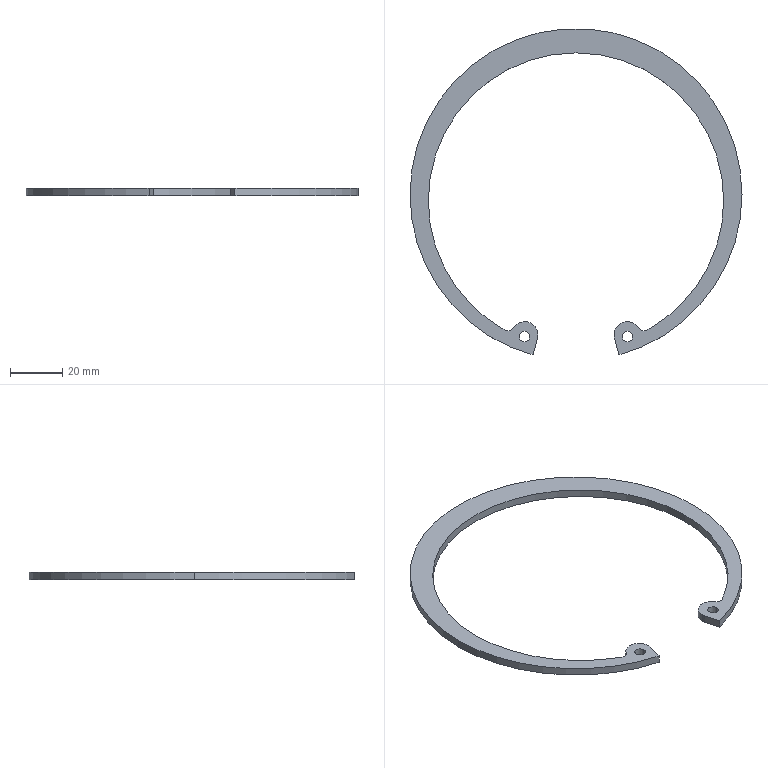Part | SolidWorks | features Extrusion 1 | 1 solid | 19 faces | box 127 x 124.836 x 3 mm | volume 7725 mm3 | cylinder 15 | plane 4 | commonest cylinder face diameters 4 x4 10 x3 113 x3 127 x3 5 x2
STEP:
#1=CARTESIAN_POINT('',(17.733,-54.327,1.5));
#2=VERTEX_POINT('',#1);
#3=CARTESIAN_POINT('',(21.733,-54.327,1.5));
#4=VERTEX_POINT('',#3);
#5=CARTESIAN_POINT('',(19.733,-54.327,1.5));
#6=DIRECTION('',(0.,0.,1.));
#7=DIRECTION('',(-1.,0.,0.));
#8=AXIS2_PLACEMENT_3D('',#5,#6,#7);
#9=CIRCLE('',#8,2.);
#10=EDGE_CURVE('',#2,#4,#9,.T.);
#11=ORIENTED_EDGE('',*,*,#10,.T.);
#12=CARTESIAN_POINT('',(21.733,-54.327,-1.5));
#13=VERTEX_POINT('',#12);
#14=CARTESIAN_POINT('',(21.733,-54.327,1.5));
#15=DIRECTION('',(0.,0.,-1.));
#16=VECTOR('',#15,1000.);
#17=LINE('',#14,#16);
#18=EDGE_CURVE('',#4,#13,#17,.T.);
#19=ORIENTED_EDGE('',*,*,#18,.T.);
#20=CARTESIAN_POINT('',(17.733,-54.327,-1.5));
#21=VERTEX_POINT('',#20);
#22=CARTESIAN_POINT('',(19.733,-54.327,-1.5));
#23=DIRECTION('',(0.,0.,1.));
#24=DIRECTION('',(-1.,0.,0.));
#25=AXIS2_PLACEMENT_3D('',#22,#23,#24);
#26=CIRCLE('',#25,2.);
#27=EDGE_CURVE('',#21,#13,#26,.T.);
#28=ORIENTED_EDGE('',*,*,#27,.F.);
#29=CARTESIAN_POINT('',(17.733,-54.327,1.5));
#30=DIRECTION('',(0.,0.,-1.));
#31=VECTOR('',#30,1000.);
#32=LINE('',#29,#31);
#33=EDGE_CURVE('',#2,#21,#32,.T.);
#34=ORIENTED_EDGE('',*,*,#33,.F.);
#35=EDGE_LOOP('',(#11,#19,#28,#34));
#36=FACE_OUTER_BOUND('',#35,.T.);
#37=CARTESIAN_POINT('',(19.733,-54.327,1.5));
#38=DIRECTION('',(0.,0.,-1.));
#39=DIRECTION('',(-1.,0.,0.));
#40=AXIS2_PLACEMENT_3D('',#37,#38,#39);
#41=CYLINDRICAL_SURFACE('',#40,2.);
#42=ADVANCED_FACE('',(#36),#41,.F.);
#43=CARTESIAN_POINT('',(-21.733,-54.327,1.5));
#44=VERTEX_POINT('',#43);
#45=CARTESIAN_POINT('',(-17.733,-54.327,1.5));
#46=VERTEX_POINT('',#45);
#47=CARTESIAN_POINT('',(-19.733,-54.327,1.5));
#48=DIRECTION('',(0.,0.,1.));
#49=DIRECTION('',(1.,0.,0.));
#50=AXIS2_PLACEMENT_3D('',#47,#48,#49);
#51=CIRCLE('',#50,2.);
#52=EDGE_CURVE('',#44,#46,#51,.T.);
#53=ORIENTED_EDGE('',*,*,#52,.T.);
#54=CARTESIAN_POINT('',(-17.733,-54.327,-1.5));
#55=VERTEX_POINT('',#54);
#56=CARTESIAN_POINT('',(-17.733,-54.327,1.5));
#57=DIRECTION('',(0.,0.,-1.));
#58=VECTOR('',#57,1000.);
#59=LINE('',#56,#58);
#60=EDGE_CURVE('',#46,#55,#59,.T.);
#61=ORIENTED_EDGE('',*,*,#60,.T.);
#62=CARTESIAN_POINT('',(-21.733,-54.327,-1.5));
#63=VERTEX_POINT('',#62);
#64=CARTESIAN_POINT('',(-19.733,-54.327,-1.5));
#65=DIRECTION('',(0.,0.,1.));
#66=DIRECTION('',(1.,0.,0.));
#67=AXIS2_PLACEMENT_3D('',#64,#65,#66);
#68=CIRCLE('',#67,2.);
#69=EDGE_CURVE('',#63,#55,#68,.T.);
#70=ORIENTED_EDGE('',*,*,#69,.F.);
#71=CARTESIAN_POINT('',(-21.733,-54.327,1.5));
#72=DIRECTION('',(0.,0.,-1.));
#73=VECTOR('',#72,1000.);
#74=LINE('',#71,#73);
#75=EDGE_CURVE('',#44,#63,#74,.T.);
#76=ORIENTED_EDGE('',*,*,#75,.F.);
#77=EDGE_LOOP('',(#53,#61,#70,#76));
#78=FACE_OUTER_BOUND('',#77,.T.);
#79=CARTESIAN_POINT('',(-19.733,-54.327,1.5));
#80=DIRECTION('',(0.,0.,-1.));
#81=DIRECTION('',(-1.,0.,0.));
#82=AXIS2_PLACEMENT_3D('',#79,#80,#81);
#83=CYLINDRICAL_SURFACE('',#82,2.);
#84=ADVANCED_FACE('',(#78),#83,.F.);
#85=CARTESIAN_POINT('',(63.5,0.,1.5));
#86=VERTEX_POINT('',#85);
#87=CARTESIAN_POINT('',(-63.5,0.,1.5));
#88=VERTEX_POINT('',#87);
#89=CARTESIAN_POINT('',(0.,0.,1.5));
#90=DIRECTION('',(0.,0.,1.));
#91=DIRECTION('',(1.,0.,0.));
#92=AXIS2_PLACEMENT_3D('',#89,#90,#91);
#93=CIRCLE('',#92,63.5);
#94=EDGE_CURVE('',#86,#88,#93,.T.);
#95=ORIENTED_EDGE('',*,*,#94,.F.);
#96=CARTESIAN_POINT('',(63.5,0.,-1.5));
#97=VERTEX_POINT('',#96);
#98=CARTESIAN_POINT('',(63.5,0.,1.5));
#99=DIRECTION('',(0.,0.,-1.));
#100=VECTOR('',#99,1000.);
#101=LINE('',#98,#100);
#102=EDGE_CURVE('',#86,#97,#101,.T.);
#103=ORIENTED_EDGE('',*,*,#102,.T.);
#104=CARTESIAN_POINT('',(-63.5,0.,-1.5));
#105=VERTEX_POINT('',#104);
#106=CARTESIAN_POINT('',(0.,0.,-1.5));
#107=DIRECTION('',(0.,0.,1.));
#108=DIRECTION('',(1.,0.,0.));
#109=AXIS2_PLACEMENT_3D('',#106,#107,#108);
#110=CIRCLE('',#109,63.5);
#111=EDGE_CURVE('',#97,#105,#110,.T.);
#112=ORIENTED_EDGE('',*,*,#111,.T.);
#113=CARTESIAN_POINT('',(-63.5,0.,1.5));
#114=DIRECTION('',(0.,0.,-1.));
#115=VECTOR('',#114,1000.);
#116=LINE('',#113,#115);
#117=EDGE_CURVE('',#88,#105,#116,.T.);
#118=ORIENTED_EDGE('',*,*,#117,.F.);
#119=EDGE_LOOP('',(#95,#103,#112,#118));
#120=FACE_OUTER_BOUND('',#119,.T.);
#121=CARTESIAN_POINT('',(0.,0.,1.5));
#122=DIRECTION('',(0.,0.,-1.));
#123=DIRECTION('',(-1.,0.,0.));
#124=AXIS2_PLACEMENT_3D('',#121,#122,#123);
#125=CYLINDRICAL_SURFACE('',#124,63.5);
#126=ADVANCED_FACE('',(#120),#125,.T.);
#127=CARTESIAN_POINT('',(-16.435,-61.336,1.5));
#128=VERTEX_POINT('',#127);
#129=CARTESIAN_POINT('',(0.,0.,1.5));
#130=DIRECTION('',(0.,0.,1.));
#131=DIRECTION('',(1.,0.,0.));
#132=AXIS2_PLACEMENT_3D('',#129,#130,#131);
#133=CIRCLE('',#132,63.5);
#134=EDGE_CURVE('',#88,#128,#133,.T.);
#135=ORIENTED_EDGE('',*,*,#134,.F.);
#136=ORIENTED_EDGE('',*,*,#117,.T.);
#137=CARTESIAN_POINT('',(-16.435,-61.336,-1.5));
#138=VERTEX_POINT('',#137);
#139=CARTESIAN_POINT('',(0.,0.,-1.5));
#140=DIRECTION('',(0.,0.,1.));
#141=DIRECTION('',(1.,0.,0.));
#142=AXIS2_PLACEMENT_3D('',#139,#140,#141);
#143=CIRCLE('',#142,63.5);
#144=EDGE_CURVE('',#105,#138,#143,.T.);
#145=ORIENTED_EDGE('',*,*,#144,.T.);
#146=CARTESIAN_POINT('',(-16.435,-61.336,1.5));
#147=DIRECTION('',(0.,0.,-1.));
#148=VECTOR('',#147,1000.);
#149=LINE('',#146,#148);
#150=EDGE_CURVE('',#128,#138,#149,.T.);
#151=ORIENTED_EDGE('',*,*,#150,.F.);
#152=EDGE_LOOP('',(#135,#136,#145,#151));
#153=FACE_OUTER_BOUND('',#152,.T.);
#154=CARTESIAN_POINT('',(0.,0.,1.5));
#155=DIRECTION('',(0.,0.,-1.));
#156=DIRECTION('',(-1.,0.,0.));
#157=AXIS2_PLACEMENT_3D('',#154,#155,#156);
#158=CYLINDRICAL_SURFACE('',#157,63.5);
#159=ADVANCED_FACE('',(#153),#158,.T.);
#160=CARTESIAN_POINT('',(14.538,-53.6,1.5));
#161=VERTEX_POINT('',#160);
#162=CARTESIAN_POINT('',(14.709,-54.894,1.5));
#163=VERTEX_POINT('',#162);
#164=CARTESIAN_POINT('',(19.538,-53.6,1.5));
#165=DIRECTION('',(0.,0.,1.));
#166=DIRECTION('',(-1.,0.,0.));
#167=AXIS2_PLACEMENT_3D('',#164,#165,#166);
#168=CIRCLE('',#167,5.);
#169=EDGE_CURVE('',#161,#163,#168,.T.);
#170=ORIENTED_EDGE('',*,*,#169,.F.);
#171=CARTESIAN_POINT('',(14.538,-53.6,-1.5));
#172=VERTEX_POINT('',#171);
#173=CARTESIAN_POINT('',(14.538,-53.6,1.5));
#174=DIRECTION('',(0.,0.,-1.));
#175=VECTOR('',#174,1000.);
#176=LINE('',#173,#175);
#177=EDGE_CURVE('',#161,#172,#176,.T.);
#178=ORIENTED_EDGE('',*,*,#177,.T.);
#179=CARTESIAN_POINT('',(14.709,-54.894,-1.5));
#180=VERTEX_POINT('',#179);
#181=CARTESIAN_POINT('',(19.538,-53.6,-1.5));
#182=DIRECTION('',(0.,0.,1.));
#183=DIRECTION('',(-1.,0.,0.));
#184=AXIS2_PLACEMENT_3D('',#181,#182,#183);
#185=CIRCLE('',#184,5.);
#186=EDGE_CURVE('',#172,#180,#185,.T.);
#187=ORIENTED_EDGE('',*,*,#186,.T.);
#188=CARTESIAN_POINT('',(14.709,-54.894,1.5));
#189=DIRECTION('',(0.,0.,-1.));
#190=VECTOR('',#189,1000.);
#191=LINE('',#188,#190);
#192=EDGE_CURVE('',#163,#180,#191,.T.);
#193=ORIENTED_EDGE('',*,*,#192,.F.);
#194=EDGE_LOOP('',(#170,#178,#187,#193));
#195=FACE_OUTER_BOUND('',#194,.T.);
#196=CARTESIAN_POINT('',(19.538,-53.6,1.5));
#197=DIRECTION('',(0.,0.,-1.));
#198=DIRECTION('',(-1.,0.,0.));
#199=AXIS2_PLACEMENT_3D('',#196,#197,#198);
#200=CYLINDRICAL_SURFACE('',#199,5.);
#201=ADVANCED_FACE('',(#195),#200,.T.);
#202=CARTESIAN_POINT('',(56.5,-2.3,1.5));
#203=VERTEX_POINT('',#202);
#204=CARTESIAN_POINT('',(27.126,-51.862,1.5));
#205=VERTEX_POINT('',#204);
#206=CARTESIAN_POINT('',(0.,-2.3,1.5));
#207=DIRECTION('',(0.,0.,-1.));
#208=DIRECTION('',(1.,0.,0.));
#209=AXIS2_PLACEMENT_3D('',#206,#207,#208);
#210=CIRCLE('',#209,56.5);
#211=EDGE_CURVE('',#203,#205,#210,.T.);
#212=ORIENTED_EDGE('',*,*,#211,.F.);
#213=CARTESIAN_POINT('',(56.5,-2.3,-1.5));
#214=VERTEX_POINT('',#213);
#215=CARTESIAN_POINT('',(56.5,-2.3,1.5));
#216=DIRECTION('',(0.,0.,-1.));
#217=VECTOR('',#216,1000.);
#218=LINE('',#215,#217);
#219=EDGE_CURVE('',#203,#214,#218,.T.);
#220=ORIENTED_EDGE('',*,*,#219,.T.);
#221=CARTESIAN_POINT('',(27.126,-51.862,-1.5));
#222=VERTEX_POINT('',#221);
#223=CARTESIAN_POINT('',(0.,-2.3,-1.5));
#224=DIRECTION('',(0.,0.,-1.));
#225=DIRECTION('',(1.,0.,0.));
#226=AXIS2_PLACEMENT_3D('',#223,#224,#225);
#227=CIRCLE('',#226,56.5);
#228=EDGE_CURVE('',#214,#222,#227,.T.);
#229=ORIENTED_EDGE('',*,*,#228,.T.);
#230=CARTESIAN_POINT('',(27.126,-51.862,1.5));
#231=DIRECTION('',(0.,0.,-1.));
#232=VECTOR('',#231,1000.);
#233=LINE('',#230,#232);
#234=EDGE_CURVE('',#205,#222,#233,.T.);
#235=ORIENTED_EDGE('',*,*,#234,.F.);
#236=EDGE_LOOP('',(#212,#220,#229,#235));
#237=FACE_OUTER_BOUND('',#236,.T.);
#238=CARTESIAN_POINT('',(0.,-2.3,1.5));
#239=DIRECTION('',(0.,0.,-1.));
#240=DIRECTION('',(-1.,0.,0.));
#241=AXIS2_PLACEMENT_3D('',#238,#239,#240);
#242=CYLINDRICAL_SURFACE('',#241,56.5);
#243=ADVANCED_FACE('',(#237),#242,.F.);
#244=ORIENTED_EDGE('',*,*,#219,.F.);
#245=CARTESIAN_POINT('',(-56.5,-2.3,1.5));
#246=VERTEX_POINT('',#245);
#247=CARTESIAN_POINT('',(0.,-2.3,1.5));
#248=DIRECTION('',(0.,0.,-1.));
#249=DIRECTION('',(1.,0.,0.));
#250=AXIS2_PLACEMENT_3D('',#247,#248,#249);
#251=CIRCLE('',#250,56.5);
#252=EDGE_CURVE('',#246,#203,#251,.T.);
#253=ORIENTED_EDGE('',*,*,#252,.F.);
#254=CARTESIAN_POINT('',(-56.5,-2.3,-1.5));
#255=VERTEX_POINT('',#254);
#256=CARTESIAN_POINT('',(-56.5,-2.3,1.5));
#257=DIRECTION('',(0.,0.,-1.));
#258=VECTOR('',#257,1000.);
#259=LINE('',#256,#258);
#260=EDGE_CURVE('',#246,#255,#259,.T.);
#261=ORIENTED_EDGE('',*,*,#260,.T.);
#262=CARTESIAN_POINT('',(0.,-2.3,-1.5));
#263=DIRECTION('',(0.,0.,-1.));
#264=DIRECTION('',(1.,0.,0.));
#265=AXIS2_PLACEMENT_3D('',#262,#263,#264);
#266=CIRCLE('',#265,56.5);
#267=EDGE_CURVE('',#255,#214,#266,.T.);
#268=ORIENTED_EDGE('',*,*,#267,.T.);
#269=EDGE_LOOP('',(#244,#253,#261,#268));
#270=FACE_OUTER_BOUND('',#269,.T.);
#271=CARTESIAN_POINT('',(0.,-2.3,1.5));
#272=DIRECTION('',(0.,0.,-1.));
#273=DIRECTION('',(-1.,0.,0.));
#274=AXIS2_PLACEMENT_3D('',#271,#272,#273);
#275=CYLINDRICAL_SURFACE('',#274,56.5);
#276=ADVANCED_FACE('',(#270),#275,.F.);
#277=ORIENTED_EDGE('',*,*,#52,.F.);
#278=CARTESIAN_POINT('',(-19.733,-54.327,1.5));
#279=DIRECTION('',(0.,0.,1.));
#280=DIRECTION('',(1.,0.,0.));
#281=AXIS2_PLACEMENT_3D('',#278,#279,#280);
#282=CIRCLE('',#281,2.);
#283=EDGE_CURVE('',#46,#44,#282,.T.);
#284=ORIENTED_EDGE('',*,*,#283,.F.);
#285=EDGE_LOOP('',(#277,#284));
#286=FACE_BOUND('',#285,.T.);
#287=CARTESIAN_POINT('',(-14.709,-54.894,1.5));
#288=VERTEX_POINT('',#287);
#289=CARTESIAN_POINT('',(-23.797,-50.979,1.5));
#290=VERTEX_POINT('',#289);
#291=CARTESIAN_POINT('',(-19.538,-53.6,1.5));
#292=DIRECTION('',(0.,0.,1.));
#293=DIRECTION('',(1.,0.,0.));
#294=AXIS2_PLACEMENT_3D('',#291,#292,#293);
#295=CIRCLE('',#294,5.);
#296=EDGE_CURVE('',#288,#290,#295,.T.);
#297=ORIENTED_EDGE('',*,*,#296,.T.);
#298=CARTESIAN_POINT('',(-27.126,-51.862,1.5));
#299=VERTEX_POINT('',#298);
#300=CARTESIAN_POINT('',(-25.926,-49.669,1.5));
#301=DIRECTION('',(0.,0.,-1.));
#302=DIRECTION('',(-1.,0.,0.));
#303=AXIS2_PLACEMENT_3D('',#300,#301,#302);
#304=CIRCLE('',#303,2.5);
#305=EDGE_CURVE('',#290,#299,#304,.T.);
#306=ORIENTED_EDGE('',*,*,#305,.T.);
#307=CARTESIAN_POINT('',(0.,-2.3,1.5));
#308=DIRECTION('',(0.,0.,-1.));
#309=DIRECTION('',(1.,0.,0.));
#310=AXIS2_PLACEMENT_3D('',#307,#308,#309);
#311=CIRCLE('',#310,56.5);
#312=EDGE_CURVE('',#299,#246,#311,.T.);
#313=ORIENTED_EDGE('',*,*,#312,.T.);
#314=ORIENTED_EDGE('',*,*,#252,.T.);
#315=ORIENTED_EDGE('',*,*,#211,.T.);
#316=CARTESIAN_POINT('',(23.797,-50.979,1.5));
#317=VERTEX_POINT('',#316);
#318=CARTESIAN_POINT('',(25.926,-49.669,1.5));
#319=DIRECTION('',(0.,0.,-1.));
#320=DIRECTION('',(1.,0.,0.));
#321=AXIS2_PLACEMENT_3D('',#318,#319,#320);
#322=CIRCLE('',#321,2.5);
#323=EDGE_CURVE('',#205,#317,#322,.T.);
#324=ORIENTED_EDGE('',*,*,#323,.T.);
#325=CARTESIAN_POINT('',(19.538,-53.6,1.5));
#326=DIRECTION('',(0.,0.,1.));
#327=DIRECTION('',(-1.,0.,0.));
#328=AXIS2_PLACEMENT_3D('',#325,#326,#327);
#329=CIRCLE('',#328,5.);
#330=EDGE_CURVE('',#317,#161,#329,.T.);
#331=ORIENTED_EDGE('',*,*,#330,.T.);
#332=ORIENTED_EDGE('',*,*,#169,.T.);
#333=CARTESIAN_POINT('',(16.435,-61.336,1.5));
#334=VERTEX_POINT('',#333);
#335=CARTESIAN_POINT('',(14.709,-54.894,1.5));
#336=DIRECTION('',(0.2588,-0.9659,0.));
#337=VECTOR('',#336,1000.);
#338=LINE('',#335,#337);
#339=EDGE_CURVE('',#163,#334,#338,.T.);
#340=ORIENTED_EDGE('',*,*,#339,.T.);
#341=CARTESIAN_POINT('',(0.,0.,1.5));
#342=DIRECTION('',(0.,0.,1.));
#343=DIRECTION('',(1.,0.,0.));
#344=AXIS2_PLACEMENT_3D('',#341,#342,#343);
#345=CIRCLE('',#344,63.5);
#346=EDGE_CURVE('',#334,#86,#345,.T.);
#347=ORIENTED_EDGE('',*,*,#346,.T.);
#348=ORIENTED_EDGE('',*,*,#94,.T.);
#349=ORIENTED_EDGE('',*,*,#134,.T.);
#350=CARTESIAN_POINT('',(-14.709,-54.894,1.5));
#351=DIRECTION('',(0.2588,0.9659,0.));
#352=VECTOR('',#351,1000.);
#353=LINE('',#350,#352);
#354=EDGE_CURVE('',#128,#288,#353,.T.);
#355=ORIENTED_EDGE('',*,*,#354,.T.);
#356=EDGE_LOOP('',(#297,#306,#313,#314,#315,#324,#331,#332,#340,#347,#348,#349,#355));
#357=FACE_OUTER_BOUND('',#356,.T.);
#358=ORIENTED_EDGE('',*,*,#10,.F.);
#359=CARTESIAN_POINT('',(19.733,-54.327,1.5));
#360=DIRECTION('',(0.,0.,1.));
#361=DIRECTION('',(-1.,0.,0.));
#362=AXIS2_PLACEMENT_3D('',#359,#360,#361);
#363=CIRCLE('',#362,2.);
#364=EDGE_CURVE('',#4,#2,#363,.T.);
#365=ORIENTED_EDGE('',*,*,#364,.F.);
#366=EDGE_LOOP('',(#358,#365));
#367=FACE_BOUND('',#366,.T.);
#368=CARTESIAN_POINT('',(-19.538,-53.6,1.5));
#369=DIRECTION('',(0.,0.,1.));
#370=DIRECTION('',(1.,0.,0.));
#371=AXIS2_PLACEMENT_3D('',#368,#369,#370);
#372=PLANE('',#371);
#373=ADVANCED_FACE('',(#286,#357,#367),#372,.T.);
#374=CARTESIAN_POINT('',(-14.709,-54.894,-1.5));
#375=VERTEX_POINT('',#374);
#376=CARTESIAN_POINT('',(-14.709,-54.894,1.5));
#377=DIRECTION('',(0.,0.,-1.));
#378=VECTOR('',#377,1000.);
#379=LINE('',#376,#378);
#380=EDGE_CURVE('',#288,#375,#379,.T.);
#381=ORIENTED_EDGE('',*,*,#380,.T.);
#382=CARTESIAN_POINT('',(-23.797,-50.979,-1.5));
#383=VERTEX_POINT('',#382);
#384=CARTESIAN_POINT('',(-19.538,-53.6,-1.5));
#385=DIRECTION('',(0.,0.,1.));
#386=DIRECTION('',(1.,0.,0.));
#387=AXIS2_PLACEMENT_3D('',#384,#385,#386);
#388=CIRCLE('',#387,5.);
#389=EDGE_CURVE('',#375,#383,#388,.T.);
#390=ORIENTED_EDGE('',*,*,#389,.T.);
#391=CARTESIAN_POINT('',(-23.797,-50.979,1.5));
#392=DIRECTION('',(0.,0.,-1.));
#393=VECTOR('',#392,1000.);
#394=LINE('',#391,#393);
#395=EDGE_CURVE('',#290,#383,#394,.T.);
#396=ORIENTED_EDGE('',*,*,#395,.F.);
#397=ORIENTED_EDGE('',*,*,#296,.F.);
#398=EDGE_LOOP('',(#381,#390,#396,#397));
#399=FACE_OUTER_BOUND('',#398,.T.);
#400=CARTESIAN_POINT('',(-19.538,-53.6,1.5));
#401=DIRECTION('',(0.,0.,-1.));
#402=DIRECTION('',(-1.,0.,0.));
#403=AXIS2_PLACEMENT_3D('',#400,#401,#402);
#404=CYLINDRICAL_SURFACE('',#403,5.);
#405=ADVANCED_FACE('',(#399),#404,.T.);
#406=ORIENTED_EDGE('',*,*,#395,.T.);
#407=CARTESIAN_POINT('',(-27.126,-51.862,-1.5));
#408=VERTEX_POINT('',#407);
#409=CARTESIAN_POINT('',(-25.926,-49.669,-1.5));
#410=DIRECTION('',(0.,0.,-1.));
#411=DIRECTION('',(-1.,0.,0.));
#412=AXIS2_PLACEMENT_3D('',#409,#410,#411);
#413=CIRCLE('',#412,2.5);
#414=EDGE_CURVE('',#383,#408,#413,.T.);
#415=ORIENTED_EDGE('',*,*,#414,.T.);
#416=CARTESIAN_POINT('',(-27.126,-51.862,1.5));
#417=DIRECTION('',(0.,0.,-1.));
#418=VECTOR('',#417,1000.);
#419=LINE('',#416,#418);
#420=EDGE_CURVE('',#299,#408,#419,.T.);
#421=ORIENTED_EDGE('',*,*,#420,.F.);
#422=ORIENTED_EDGE('',*,*,#305,.F.);
#423=EDGE_LOOP('',(#406,#415,#421,#422));
#424=FACE_OUTER_BOUND('',#423,.T.);
#425=CARTESIAN_POINT('',(-25.926,-49.669,1.5));
#426=DIRECTION('',(0.,0.,-1.));
#427=DIRECTION('',(-1.,0.,0.));
#428=AXIS2_PLACEMENT_3D('',#425,#426,#427);
#429=CYLINDRICAL_SURFACE('',#428,2.5);
#430=ADVANCED_FACE('',(#424),#429,.F.);
#431=ORIENTED_EDGE('',*,*,#260,.F.);
#432=ORIENTED_EDGE('',*,*,#312,.F.);
#433=ORIENTED_EDGE('',*,*,#420,.T.);
#434=CARTESIAN_POINT('',(0.,-2.3,-1.5));
#435=DIRECTION('',(0.,0.,-1.));
#436=DIRECTION('',(1.,0.,0.));
#437=AXIS2_PLACEMENT_3D('',#434,#435,#436);
#438=CIRCLE('',#437,56.5);
#439=EDGE_CURVE('',#408,#255,#438,.T.);
#440=ORIENTED_EDGE('',*,*,#439,.T.);
#441=EDGE_LOOP('',(#431,#432,#433,#440));
#442=FACE_OUTER_BOUND('',#441,.T.);
#443=CARTESIAN_POINT('',(0.,-2.3,1.5));
#444=DIRECTION('',(0.,0.,-1.));
#445=DIRECTION('',(-1.,0.,0.));
#446=AXIS2_PLACEMENT_3D('',#443,#444,#445);
#447=CYLINDRICAL_SURFACE('',#446,56.5);
#448=ADVANCED_FACE('',(#442),#447,.F.);
#449=ORIENTED_EDGE('',*,*,#234,.T.);
#450=CARTESIAN_POINT('',(23.797,-50.979,-1.5));
#451=VERTEX_POINT('',#450);
#452=CARTESIAN_POINT('',(25.926,-49.669,-1.5));
#453=DIRECTION('',(0.,0.,-1.));
#454=DIRECTION('',(1.,0.,0.));
#455=AXIS2_PLACEMENT_3D('',#452,#453,#454);
#456=CIRCLE('',#455,2.5);
#457=EDGE_CURVE('',#222,#451,#456,.T.);
#458=ORIENTED_EDGE('',*,*,#457,.T.);
#459=CARTESIAN_POINT('',(23.797,-50.979,1.5));
#460=DIRECTION('',(0.,0.,-1.));
#461=VECTOR('',#460,1000.);
#462=LINE('',#459,#461);
#463=EDGE_CURVE('',#317,#451,#462,.T.);
#464=ORIENTED_EDGE('',*,*,#463,.F.);
#465=ORIENTED_EDGE('',*,*,#323,.F.);
#466=EDGE_LOOP('',(#449,#458,#464,#465));
#467=FACE_OUTER_BOUND('',#466,.T.);
#468=CARTESIAN_POINT('',(25.926,-49.669,1.5));
#469=DIRECTION('',(0.,0.,-1.));
#470=DIRECTION('',(-1.,0.,0.));
#471=AXIS2_PLACEMENT_3D('',#468,#469,#470);
#472=CYLINDRICAL_SURFACE('',#471,2.5);
#473=ADVANCED_FACE('',(#467),#472,.F.);
#474=ORIENTED_EDGE('',*,*,#177,.F.);
#475=ORIENTED_EDGE('',*,*,#330,.F.);
#476=ORIENTED_EDGE('',*,*,#463,.T.);
#477=CARTESIAN_POINT('',(19.538,-53.6,-1.5));
#478=DIRECTION('',(0.,0.,1.));
#479=DIRECTION('',(-1.,0.,0.));
#480=AXIS2_PLACEMENT_3D('',#477,#478,#479);
#481=CIRCLE('',#480,5.);
#482=EDGE_CURVE('',#451,#172,#481,.T.);
#483=ORIENTED_EDGE('',*,*,#482,.T.);
#484=EDGE_LOOP('',(#474,#475,#476,#483));
#485=FACE_OUTER_BOUND('',#484,.T.);
#486=CARTESIAN_POINT('',(19.538,-53.6,1.5));
#487=DIRECTION('',(0.,0.,-1.));
#488=DIRECTION('',(-1.,0.,0.));
#489=AXIS2_PLACEMENT_3D('',#486,#487,#488);
#490=CYLINDRICAL_SURFACE('',#489,5.);
#491=ADVANCED_FACE('',(#485),#490,.T.);
#492=ORIENTED_EDGE('',*,*,#192,.T.);
#493=CARTESIAN_POINT('',(16.435,-61.336,-1.5));
#494=VERTEX_POINT('',#493);
#495=CARTESIAN_POINT('',(14.709,-54.894,-1.5));
#496=DIRECTION('',(0.2588,-0.9659,0.));
#497=VECTOR('',#496,1000.);
#498=LINE('',#495,#497);
#499=EDGE_CURVE('',#180,#494,#498,.T.);
#500=ORIENTED_EDGE('',*,*,#499,.T.);
#501=CARTESIAN_POINT('',(16.435,-61.336,1.5));
#502=DIRECTION('',(0.,0.,-1.));
#503=VECTOR('',#502,1000.);
#504=LINE('',#501,#503);
#505=EDGE_CURVE('',#334,#494,#504,.T.);
#506=ORIENTED_EDGE('',*,*,#505,.F.);
#507=ORIENTED_EDGE('',*,*,#339,.F.);
#508=EDGE_LOOP('',(#492,#500,#506,#507));
#509=FACE_OUTER_BOUND('',#508,.T.);
#510=CARTESIAN_POINT('',(14.709,-54.894,1.5));
#511=DIRECTION('',(0.9659,0.2588,0.));
#512=DIRECTION('',(-0.2588,0.9659,0.));
#513=AXIS2_PLACEMENT_3D('',#510,#511,#512);
#514=PLANE('',#513);
#515=ADVANCED_FACE('',(#509),#514,.F.);
#516=ORIENTED_EDGE('',*,*,#102,.F.);
#517=ORIENTED_EDGE('',*,*,#346,.F.);
#518=ORIENTED_EDGE('',*,*,#505,.T.);
#519=CARTESIAN_POINT('',(0.,0.,-1.5));
#520=DIRECTION('',(0.,0.,1.));
#521=DIRECTION('',(1.,0.,0.));
#522=AXIS2_PLACEMENT_3D('',#519,#520,#521);
#523=CIRCLE('',#522,63.5);
#524=EDGE_CURVE('',#494,#97,#523,.T.);
#525=ORIENTED_EDGE('',*,*,#524,.T.);
#526=EDGE_LOOP('',(#516,#517,#518,#525));
#527=FACE_OUTER_BOUND('',#526,.T.);
#528=CARTESIAN_POINT('',(0.,0.,1.5));
#529=DIRECTION('',(0.,0.,-1.));
#530=DIRECTION('',(-1.,0.,0.));
#531=AXIS2_PLACEMENT_3D('',#528,#529,#530);
#532=CYLINDRICAL_SURFACE('',#531,63.5);
#533=ADVANCED_FACE('',(#527),#532,.T.);
#534=ORIENTED_EDGE('',*,*,#150,.T.);
#535=CARTESIAN_POINT('',(-14.709,-54.894,-1.5));
#536=DIRECTION('',(0.2588,0.9659,0.));
#537=VECTOR('',#536,1000.);
#538=LINE('',#535,#537);
#539=EDGE_CURVE('',#138,#375,#538,.T.);
#540=ORIENTED_EDGE('',*,*,#539,.T.);
#541=ORIENTED_EDGE('',*,*,#380,.F.);
#542=ORIENTED_EDGE('',*,*,#354,.F.);
#543=EDGE_LOOP('',(#534,#540,#541,#542));
#544=FACE_OUTER_BOUND('',#543,.T.);
#545=CARTESIAN_POINT('',(-14.709,-54.894,1.5));
#546=DIRECTION('',(-0.9659,0.2588,0.));
#547=DIRECTION('',(-0.2588,-0.9659,0.));
#548=AXIS2_PLACEMENT_3D('',#545,#546,#547);
#549=PLANE('',#548);
#550=ADVANCED_FACE('',(#544),#549,.F.);
#551=ORIENTED_EDGE('',*,*,#60,.F.);
#552=ORIENTED_EDGE('',*,*,#283,.T.);
#553=ORIENTED_EDGE('',*,*,#75,.T.);
#554=CARTESIAN_POINT('',(-19.733,-54.327,-1.5));
#555=DIRECTION('',(0.,0.,1.));
#556=DIRECTION('',(1.,0.,0.));
#557=AXIS2_PLACEMENT_3D('',#554,#555,#556);
#558=CIRCLE('',#557,2.);
#559=EDGE_CURVE('',#55,#63,#558,.T.);
#560=ORIENTED_EDGE('',*,*,#559,.F.);
#561=EDGE_LOOP('',(#551,#552,#553,#560));
#562=FACE_OUTER_BOUND('',#561,.T.);
#563=CARTESIAN_POINT('',(-19.733,-54.327,1.5));
#564=DIRECTION('',(0.,0.,-1.));
#565=DIRECTION('',(-1.,0.,0.));
#566=AXIS2_PLACEMENT_3D('',#563,#564,#565);
#567=CYLINDRICAL_SURFACE('',#566,2.);
#568=ADVANCED_FACE('',(#562),#567,.F.);
#569=ORIENTED_EDGE('',*,*,#18,.F.);
#570=ORIENTED_EDGE('',*,*,#364,.T.);
#571=ORIENTED_EDGE('',*,*,#33,.T.);
#572=CARTESIAN_POINT('',(19.733,-54.327,-1.5));
#573=DIRECTION('',(0.,0.,1.));
#574=DIRECTION('',(-1.,0.,0.));
#575=AXIS2_PLACEMENT_3D('',#572,#573,#574);
#576=CIRCLE('',#575,2.);
#577=EDGE_CURVE('',#13,#21,#576,.T.);
#578=ORIENTED_EDGE('',*,*,#577,.F.);
#579=EDGE_LOOP('',(#569,#570,#571,#578));
#580=FACE_OUTER_BOUND('',#579,.T.);
#581=CARTESIAN_POINT('',(19.733,-54.327,1.5));
#582=DIRECTION('',(0.,0.,-1.));
#583=DIRECTION('',(-1.,0.,0.));
#584=AXIS2_PLACEMENT_3D('',#581,#582,#583);
#585=CYLINDRICAL_SURFACE('',#584,2.);
#586=ADVANCED_FACE('',(#580),#585,.F.);
#587=ORIENTED_EDGE('',*,*,#27,.T.);
#588=ORIENTED_EDGE('',*,*,#577,.T.);
#589=EDGE_LOOP('',(#587,#588));
#590=FACE_BOUND('',#589,.T.);
#591=ORIENTED_EDGE('',*,*,#69,.T.);
#592=ORIENTED_EDGE('',*,*,#559,.T.);
#593=EDGE_LOOP('',(#591,#592));
#594=FACE_BOUND('',#593,.T.);
#595=ORIENTED_EDGE('',*,*,#389,.F.);
#596=ORIENTED_EDGE('',*,*,#539,.F.);
#597=ORIENTED_EDGE('',*,*,#144,.F.);
#598=ORIENTED_EDGE('',*,*,#111,.F.);
#599=ORIENTED_EDGE('',*,*,#524,.F.);
#600=ORIENTED_EDGE('',*,*,#499,.F.);
#601=ORIENTED_EDGE('',*,*,#186,.F.);
#602=ORIENTED_EDGE('',*,*,#482,.F.);
#603=ORIENTED_EDGE('',*,*,#457,.F.);
#604=ORIENTED_EDGE('',*,*,#228,.F.);
#605=ORIENTED_EDGE('',*,*,#267,.F.);
#606=ORIENTED_EDGE('',*,*,#439,.F.);
#607=ORIENTED_EDGE('',*,*,#414,.F.);
#608=EDGE_LOOP('',(#595,#596,#597,#598,#599,#600,#601,#602,#603,#604,#605,#606,#607));
#609=FACE_OUTER_BOUND('',#608,.T.);
#610=CARTESIAN_POINT('',(-19.538,-53.6,-1.5));
#611=DIRECTION('',(0.,0.,1.));
#612=DIRECTION('',(1.,0.,0.));
#613=AXIS2_PLACEMENT_3D('',#610,#611,#612);
#614=PLANE('',#613);
#615=ADVANCED_FACE('',(#590,#594,#609),#614,.F.);
#616=CLOSED_SHELL('',(#42,#84,#126,#159,#201,#243,#276,#373,#405,#430,#448,#473,#491,#515,#533,#550,#568,#586,#615));
#617=MANIFOLD_SOLID_BREP('',#616);
#618=CARTESIAN_POINT('',(0.,0.,0.));
#619=DIRECTION('',(0.,0.,1.));
#620=DIRECTION('',(1.,0.,0.));
#621=AXIS2_PLACEMENT_3D('',#618,#619,#620);
#622=(LENGTH_UNIT()NAMED_UNIT(*)SI_UNIT(.MILLI.,.METRE.));
#623=UNCERTAINTY_MEASURE_WITH_UNIT(LENGTH_MEASURE(0.00001),#622,'','');
#624=(NAMED_UNIT(*)PLANE_ANGLE_UNIT()SI_UNIT($,.RADIAN.));
#625=(NAMED_UNIT(*)SI_UNIT($,.STERADIAN.)SOLID_ANGLE_UNIT());
#626=(GEOMETRIC_REPRESENTATION_CONTEXT(3)GLOBAL_UNCERTAINTY_ASSIGNED_CONTEXT((#623))GLOBAL_UNIT_ASSIGNED_CONTEXT((#622,#624,#625))REPRESENTATION_CONTEXT('',''));
#627=ADVANCED_BREP_SHAPE_REPRESENTATION('',(#617,#621),#626);